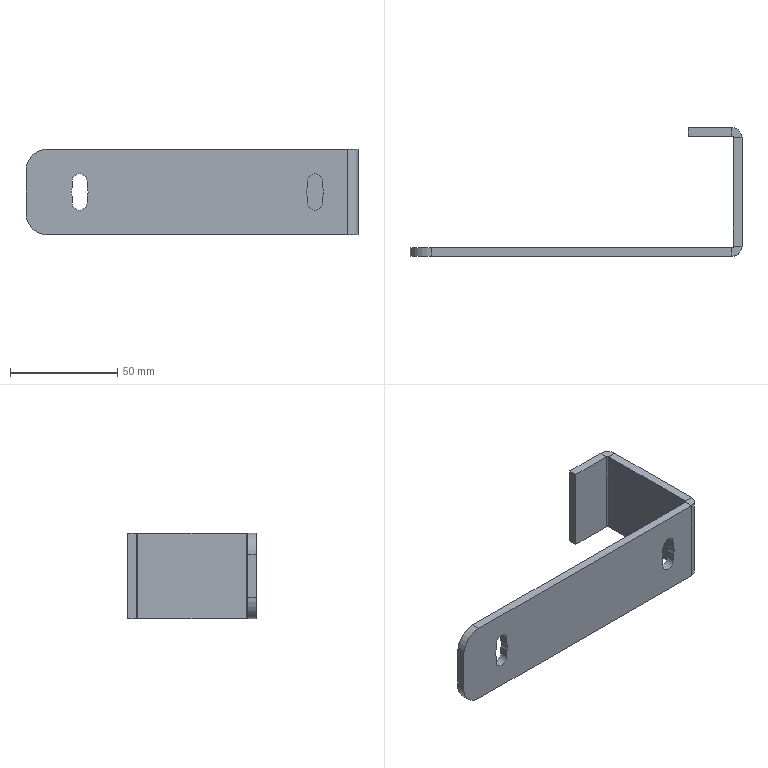Part | SolidWorks | features ICE 2, Fillet 1, FlatPattern 1, SMBaseFlange 1, SheetMetal 1 | 1 solid | 42 faces | box 155 x 60 x 40 mm | volume 35684 mm3 | plane 26 | cylinder 16 | commonest cylinder face diameters 8 x6 7 x4 1.473 x2 9.473 x2 20 x2
STEP:
#1=CARTESIAN_POINT('',(-126.,4.,0.));
#2=VERTEX_POINT('',#1);
#3=CARTESIAN_POINT('',(-126.5,4.,1.936));
#4=VERTEX_POINT('',#3);
#5=CARTESIAN_POINT('',(-130.,4.,0.));
#6=DIRECTION('',(0.,-1.,0.));
#7=DIRECTION('',(1.,0.,0.));
#8=AXIS2_PLACEMENT_3D('',#5,#6,#7);
#9=CIRCLE('',#8,4.);
#10=EDGE_CURVE('',#2,#4,#9,.T.);
#11=ORIENTED_EDGE('',*,*,#10,.F.);
#12=CARTESIAN_POINT('',(-126.,0.,0.));
#13=VERTEX_POINT('',#12);
#14=CARTESIAN_POINT('',(-126.,4.,0.));
#15=DIRECTION('',(0.,-1.,0.));
#16=VECTOR('',#15,1000.);
#17=LINE('',#14,#16);
#18=EDGE_CURVE('',#2,#13,#17,.T.);
#19=ORIENTED_EDGE('',*,*,#18,.T.);
#20=CARTESIAN_POINT('',(-126.5,0.,1.936));
#21=VERTEX_POINT('',#20);
#22=CARTESIAN_POINT('',(-130.,0.,0.));
#23=DIRECTION('',(0.,-1.,0.));
#24=DIRECTION('',(1.,0.,0.));
#25=AXIS2_PLACEMENT_3D('',#22,#23,#24);
#26=CIRCLE('',#25,4.);
#27=EDGE_CURVE('',#13,#21,#26,.T.);
#28=ORIENTED_EDGE('',*,*,#27,.T.);
#29=CARTESIAN_POINT('',(-126.5,4.,1.936));
#30=DIRECTION('',(0.,-1.,0.));
#31=VECTOR('',#30,1000.);
#32=LINE('',#29,#31);
#33=EDGE_CURVE('',#4,#21,#32,.T.);
#34=ORIENTED_EDGE('',*,*,#33,.F.);
#35=EDGE_LOOP('',(#11,#19,#28,#34));
#36=FACE_OUTER_BOUND('',#35,.T.);
#37=CARTESIAN_POINT('',(-130.,4.,0.));
#38=DIRECTION('',(0.,-1.,0.));
#39=DIRECTION('',(1.,0.,0.));
#40=AXIS2_PLACEMENT_3D('',#37,#38,#39);
#41=CYLINDRICAL_SURFACE('',#40,4.);
#42=ADVANCED_FACE('',(#36),#41,.F.);
#43=CARTESIAN_POINT('',(-16.,4.,0.));
#44=VERTEX_POINT('',#43);
#45=CARTESIAN_POINT('',(-16.5,4.,1.936));
#46=VERTEX_POINT('',#45);
#47=CARTESIAN_POINT('',(-20.,4.,0.));
#48=DIRECTION('',(0.,-1.,0.));
#49=DIRECTION('',(1.,0.,0.));
#50=AXIS2_PLACEMENT_3D('',#47,#48,#49);
#51=CIRCLE('',#50,4.);
#52=EDGE_CURVE('',#44,#46,#51,.T.);
#53=ORIENTED_EDGE('',*,*,#52,.F.);
#54=CARTESIAN_POINT('',(-16.,0.,0.));
#55=VERTEX_POINT('',#54);
#56=CARTESIAN_POINT('',(-16.,4.,0.));
#57=DIRECTION('',(0.,-1.,0.));
#58=VECTOR('',#57,1000.);
#59=LINE('',#56,#58);
#60=EDGE_CURVE('',#44,#55,#59,.T.);
#61=ORIENTED_EDGE('',*,*,#60,.T.);
#62=CARTESIAN_POINT('',(-16.5,0.,1.936));
#63=VERTEX_POINT('',#62);
#64=CARTESIAN_POINT('',(-20.,0.,0.));
#65=DIRECTION('',(0.,-1.,0.));
#66=DIRECTION('',(1.,0.,0.));
#67=AXIS2_PLACEMENT_3D('',#64,#65,#66);
#68=CIRCLE('',#67,4.);
#69=EDGE_CURVE('',#55,#63,#68,.T.);
#70=ORIENTED_EDGE('',*,*,#69,.T.);
#71=CARTESIAN_POINT('',(-16.5,4.,1.936));
#72=DIRECTION('',(0.,-1.,0.));
#73=VECTOR('',#72,1000.);
#74=LINE('',#71,#73);
#75=EDGE_CURVE('',#46,#63,#74,.T.);
#76=ORIENTED_EDGE('',*,*,#75,.F.);
#77=EDGE_LOOP('',(#53,#61,#70,#76));
#78=FACE_OUTER_BOUND('',#77,.T.);
#79=CARTESIAN_POINT('',(-20.,4.,0.));
#80=DIRECTION('',(0.,-1.,0.));
#81=DIRECTION('',(1.,0.,0.));
#82=AXIS2_PLACEMENT_3D('',#79,#80,#81);
#83=CYLINDRICAL_SURFACE('',#82,4.);
#84=ADVANCED_FACE('',(#78),#83,.F.);
#85=CARTESIAN_POINT('',(-23.5,4.,1.936));
#86=VERTEX_POINT('',#85);
#87=CARTESIAN_POINT('',(-23.5,4.,-1.936));
#88=VERTEX_POINT('',#87);
#89=CARTESIAN_POINT('',(-20.,4.,0.));
#90=DIRECTION('',(0.,-1.,0.));
#91=DIRECTION('',(1.,0.,0.));
#92=AXIS2_PLACEMENT_3D('',#89,#90,#91);
#93=CIRCLE('',#92,4.);
#94=EDGE_CURVE('',#86,#88,#93,.T.);
#95=ORIENTED_EDGE('',*,*,#94,.T.);
#96=CARTESIAN_POINT('',(-23.5,4.,-5.));
#97=VERTEX_POINT('',#96);
#98=CARTESIAN_POINT('',(-23.5,4.,-5.));
#99=DIRECTION('',(0.,0.,1.));
#100=VECTOR('',#99,1000.);
#101=LINE('',#98,#100);
#102=EDGE_CURVE('',#97,#88,#101,.T.);
#103=ORIENTED_EDGE('',*,*,#102,.F.);
#104=CARTESIAN_POINT('',(-16.5,4.,-5.));
#105=VERTEX_POINT('',#104);
#106=CARTESIAN_POINT('',(-20.,4.,-5.));
#107=DIRECTION('',(0.,1.,0.));
#108=DIRECTION('',(-1.,0.,0.));
#109=AXIS2_PLACEMENT_3D('',#106,#107,#108);
#110=CIRCLE('',#109,3.5);
#111=EDGE_CURVE('',#105,#97,#110,.T.);
#112=ORIENTED_EDGE('',*,*,#111,.F.);
#113=CARTESIAN_POINT('',(-16.5,4.,-1.936));
#114=VERTEX_POINT('',#113);
#115=CARTESIAN_POINT('',(-16.5,4.,-5.));
#116=DIRECTION('',(0.,0.,-1.));
#117=VECTOR('',#116,1000.);
#118=LINE('',#115,#117);
#119=EDGE_CURVE('',#114,#105,#118,.T.);
#120=ORIENTED_EDGE('',*,*,#119,.F.);
#121=CARTESIAN_POINT('',(-20.,4.,0.));
#122=DIRECTION('',(0.,-1.,0.));
#123=DIRECTION('',(1.,0.,0.));
#124=AXIS2_PLACEMENT_3D('',#121,#122,#123);
#125=CIRCLE('',#124,4.);
#126=EDGE_CURVE('',#114,#44,#125,.T.);
#127=ORIENTED_EDGE('',*,*,#126,.T.);
#128=ORIENTED_EDGE('',*,*,#52,.T.);
#129=CARTESIAN_POINT('',(-16.5,4.,5.));
#130=VERTEX_POINT('',#129);
#131=CARTESIAN_POINT('',(-16.5,4.,-5.));
#132=DIRECTION('',(0.,0.,-1.));
#133=VECTOR('',#132,1000.);
#134=LINE('',#131,#133);
#135=EDGE_CURVE('',#130,#46,#134,.T.);
#136=ORIENTED_EDGE('',*,*,#135,.F.);
#137=CARTESIAN_POINT('',(-23.5,4.,5.));
#138=VERTEX_POINT('',#137);
#139=CARTESIAN_POINT('',(-20.,4.,5.));
#140=DIRECTION('',(0.,1.,0.));
#141=DIRECTION('',(-1.,0.,0.));
#142=AXIS2_PLACEMENT_3D('',#139,#140,#141);
#143=CIRCLE('',#142,3.5);
#144=EDGE_CURVE('',#138,#130,#143,.T.);
#145=ORIENTED_EDGE('',*,*,#144,.F.);
#146=CARTESIAN_POINT('',(-23.5,4.,-5.));
#147=DIRECTION('',(0.,0.,1.));
#148=VECTOR('',#147,1000.);
#149=LINE('',#146,#148);
#150=EDGE_CURVE('',#86,#138,#149,.T.);
#151=ORIENTED_EDGE('',*,*,#150,.F.);
#152=EDGE_LOOP('',(#95,#103,#112,#120,#127,#128,#136,#145,#151));
#153=FACE_BOUND('',#152,.T.);
#154=CARTESIAN_POINT('',(-155.,4.,10.));
#155=VERTEX_POINT('',#154);
#156=CARTESIAN_POINT('',(-155.,4.,-10.));
#157=VERTEX_POINT('',#156);
#158=CARTESIAN_POINT('',(-155.,4.,20.));
#159=DIRECTION('',(0.,0.,-1.));
#160=VECTOR('',#159,1000.);
#161=LINE('',#158,#160);
#162=EDGE_CURVE('',#155,#157,#161,.T.);
#163=ORIENTED_EDGE('',*,*,#162,.F.);
#164=CARTESIAN_POINT('',(-145.,4.,20.));
#165=VERTEX_POINT('',#164);
#166=CARTESIAN_POINT('',(-145.,4.,10.));
#167=DIRECTION('',(0.,1.,0.));
#168=DIRECTION('',(1.,0.,0.));
#169=AXIS2_PLACEMENT_3D('',#166,#167,#168);
#170=CIRCLE('',#169,10.);
#171=EDGE_CURVE('',#155,#165,#170,.T.);
#172=ORIENTED_EDGE('',*,*,#171,.T.);
#173=CARTESIAN_POINT('',(-4.737,4.,20.));
#174=VERTEX_POINT('',#173);
#175=CARTESIAN_POINT('',(0.,4.,20.));
#176=DIRECTION('',(-1.,0.,0.));
#177=VECTOR('',#176,1000.);
#178=LINE('',#175,#177);
#179=EDGE_CURVE('',#174,#165,#178,.T.);
#180=ORIENTED_EDGE('',*,*,#179,.F.);
#181=CARTESIAN_POINT('',(-4.737,4.,-20.));
#182=VERTEX_POINT('',#181);
#183=CARTESIAN_POINT('',(-4.737,4.,20.));
#184=DIRECTION('',(0.,0.,-1.));
#185=VECTOR('',#184,1000.);
#186=LINE('',#183,#185);
#187=EDGE_CURVE('',#174,#182,#186,.T.);
#188=ORIENTED_EDGE('',*,*,#187,.T.);
#189=CARTESIAN_POINT('',(-145.,4.,-20.));
#190=VERTEX_POINT('',#189);
#191=CARTESIAN_POINT('',(0.,4.,-20.));
#192=DIRECTION('',(-1.,0.,0.));
#193=VECTOR('',#192,1000.);
#194=LINE('',#191,#193);
#195=EDGE_CURVE('',#182,#190,#194,.T.);
#196=ORIENTED_EDGE('',*,*,#195,.T.);
#197=CARTESIAN_POINT('',(-145.,4.,-10.));
#198=DIRECTION('',(0.,1.,0.));
#199=DIRECTION('',(1.,0.,0.));
#200=AXIS2_PLACEMENT_3D('',#197,#198,#199);
#201=CIRCLE('',#200,10.);
#202=EDGE_CURVE('',#190,#157,#201,.T.);
#203=ORIENTED_EDGE('',*,*,#202,.T.);
#204=EDGE_LOOP('',(#163,#172,#180,#188,#196,#203));
#205=FACE_OUTER_BOUND('',#204,.T.);
#206=CARTESIAN_POINT('',(-126.5,4.,-1.936));
#207=VERTEX_POINT('',#206);
#208=CARTESIAN_POINT('',(-130.,4.,0.));
#209=DIRECTION('',(0.,-1.,0.));
#210=DIRECTION('',(1.,0.,0.));
#211=AXIS2_PLACEMENT_3D('',#208,#209,#210);
#212=CIRCLE('',#211,4.);
#213=EDGE_CURVE('',#207,#2,#212,.T.);
#214=ORIENTED_EDGE('',*,*,#213,.T.);
#215=ORIENTED_EDGE('',*,*,#10,.T.);
#216=CARTESIAN_POINT('',(-126.5,4.,5.));
#217=VERTEX_POINT('',#216);
#218=CARTESIAN_POINT('',(-126.5,4.,-5.));
#219=DIRECTION('',(0.,0.,-1.));
#220=VECTOR('',#219,1000.);
#221=LINE('',#218,#220);
#222=EDGE_CURVE('',#217,#4,#221,.T.);
#223=ORIENTED_EDGE('',*,*,#222,.F.);
#224=CARTESIAN_POINT('',(-133.5,4.,5.));
#225=VERTEX_POINT('',#224);
#226=CARTESIAN_POINT('',(-130.,4.,5.));
#227=DIRECTION('',(0.,1.,0.));
#228=DIRECTION('',(-1.,0.,0.));
#229=AXIS2_PLACEMENT_3D('',#226,#227,#228);
#230=CIRCLE('',#229,3.5);
#231=EDGE_CURVE('',#225,#217,#230,.T.);
#232=ORIENTED_EDGE('',*,*,#231,.F.);
#233=CARTESIAN_POINT('',(-133.5,4.,1.936));
#234=VERTEX_POINT('',#233);
#235=CARTESIAN_POINT('',(-133.5,4.,-5.));
#236=DIRECTION('',(0.,0.,1.));
#237=VECTOR('',#236,1000.);
#238=LINE('',#235,#237);
#239=EDGE_CURVE('',#234,#225,#238,.T.);
#240=ORIENTED_EDGE('',*,*,#239,.F.);
#241=CARTESIAN_POINT('',(-133.5,4.,-1.936));
#242=VERTEX_POINT('',#241);
#243=CARTESIAN_POINT('',(-130.,4.,0.));
#244=DIRECTION('',(0.,-1.,0.));
#245=DIRECTION('',(1.,0.,0.));
#246=AXIS2_PLACEMENT_3D('',#243,#244,#245);
#247=CIRCLE('',#246,4.);
#248=EDGE_CURVE('',#234,#242,#247,.T.);
#249=ORIENTED_EDGE('',*,*,#248,.T.);
#250=CARTESIAN_POINT('',(-133.5,4.,-5.));
#251=VERTEX_POINT('',#250);
#252=CARTESIAN_POINT('',(-133.5,4.,-5.));
#253=DIRECTION('',(0.,0.,1.));
#254=VECTOR('',#253,1000.);
#255=LINE('',#252,#254);
#256=EDGE_CURVE('',#251,#242,#255,.T.);
#257=ORIENTED_EDGE('',*,*,#256,.F.);
#258=CARTESIAN_POINT('',(-126.5,4.,-5.));
#259=VERTEX_POINT('',#258);
#260=CARTESIAN_POINT('',(-130.,4.,-5.));
#261=DIRECTION('',(0.,1.,0.));
#262=DIRECTION('',(-1.,0.,0.));
#263=AXIS2_PLACEMENT_3D('',#260,#261,#262);
#264=CIRCLE('',#263,3.5);
#265=EDGE_CURVE('',#259,#251,#264,.T.);
#266=ORIENTED_EDGE('',*,*,#265,.F.);
#267=CARTESIAN_POINT('',(-126.5,4.,-5.));
#268=DIRECTION('',(0.,0.,-1.));
#269=VECTOR('',#268,1000.);
#270=LINE('',#267,#269);
#271=EDGE_CURVE('',#207,#259,#270,.T.);
#272=ORIENTED_EDGE('',*,*,#271,.F.);
#273=EDGE_LOOP('',(#214,#215,#223,#232,#240,#249,#257,#266,#272));
#274=FACE_BOUND('',#273,.T.);
#275=CARTESIAN_POINT('',(0.,4.,20.));
#276=DIRECTION('',(0.,-1.,0.));
#277=DIRECTION('',(1.,0.,0.));
#278=AXIS2_PLACEMENT_3D('',#275,#276,#277);
#279=PLANE('',#278);
#280=ADVANCED_FACE('',(#153,#205,#274),#279,.F.);
#281=CARTESIAN_POINT('',(-23.5,0.,-1.936));
#282=VERTEX_POINT('',#281);
#283=CARTESIAN_POINT('',(-23.5,0.,-5.));
#284=VERTEX_POINT('',#283);
#285=CARTESIAN_POINT('',(-23.5,0.,20.));
#286=DIRECTION('',(0.,0.,-1.));
#287=VECTOR('',#286,1000.);
#288=LINE('',#285,#287);
#289=EDGE_CURVE('',#282,#284,#288,.T.);
#290=ORIENTED_EDGE('',*,*,#289,.F.);
#291=CARTESIAN_POINT('',(-23.5,0.,1.936));
#292=VERTEX_POINT('',#291);
#293=CARTESIAN_POINT('',(-20.,0.,0.));
#294=DIRECTION('',(0.,-1.,0.));
#295=DIRECTION('',(1.,0.,0.));
#296=AXIS2_PLACEMENT_3D('',#293,#294,#295);
#297=CIRCLE('',#296,4.);
#298=EDGE_CURVE('',#292,#282,#297,.T.);
#299=ORIENTED_EDGE('',*,*,#298,.F.);
#300=CARTESIAN_POINT('',(-23.5,0.,5.));
#301=VERTEX_POINT('',#300);
#302=CARTESIAN_POINT('',(-23.5,0.,20.));
#303=DIRECTION('',(0.,0.,-1.));
#304=VECTOR('',#303,1000.);
#305=LINE('',#302,#304);
#306=EDGE_CURVE('',#301,#292,#305,.T.);
#307=ORIENTED_EDGE('',*,*,#306,.F.);
#308=CARTESIAN_POINT('',(-16.5,0.,5.));
#309=VERTEX_POINT('',#308);
#310=CARTESIAN_POINT('',(-20.,0.,5.));
#311=DIRECTION('',(0.,-1.,0.));
#312=DIRECTION('',(1.,0.,0.));
#313=AXIS2_PLACEMENT_3D('',#310,#311,#312);
#314=CIRCLE('',#313,3.5);
#315=EDGE_CURVE('',#309,#301,#314,.T.);
#316=ORIENTED_EDGE('',*,*,#315,.F.);
#317=CARTESIAN_POINT('',(-16.5,0.,20.));
#318=DIRECTION('',(0.,0.,1.));
#319=VECTOR('',#318,1000.);
#320=LINE('',#317,#319);
#321=EDGE_CURVE('',#63,#309,#320,.T.);
#322=ORIENTED_EDGE('',*,*,#321,.F.);
#323=ORIENTED_EDGE('',*,*,#69,.F.);
#324=CARTESIAN_POINT('',(-16.5,0.,-1.936));
#325=VERTEX_POINT('',#324);
#326=CARTESIAN_POINT('',(-20.,0.,0.));
#327=DIRECTION('',(0.,-1.,0.));
#328=DIRECTION('',(1.,0.,0.));
#329=AXIS2_PLACEMENT_3D('',#326,#327,#328);
#330=CIRCLE('',#329,4.);
#331=EDGE_CURVE('',#325,#55,#330,.T.);
#332=ORIENTED_EDGE('',*,*,#331,.F.);
#333=CARTESIAN_POINT('',(-16.5,0.,-5.));
#334=VERTEX_POINT('',#333);
#335=CARTESIAN_POINT('',(-16.5,0.,20.));
#336=DIRECTION('',(0.,0.,1.));
#337=VECTOR('',#336,1000.);
#338=LINE('',#335,#337);
#339=EDGE_CURVE('',#334,#325,#338,.T.);
#340=ORIENTED_EDGE('',*,*,#339,.F.);
#341=CARTESIAN_POINT('',(-20.,0.,-5.));
#342=DIRECTION('',(0.,-1.,0.));
#343=DIRECTION('',(1.,0.,0.));
#344=AXIS2_PLACEMENT_3D('',#341,#342,#343);
#345=CIRCLE('',#344,3.5);
#346=EDGE_CURVE('',#284,#334,#345,.T.);
#347=ORIENTED_EDGE('',*,*,#346,.F.);
#348=EDGE_LOOP('',(#290,#299,#307,#316,#322,#323,#332,#340,#347));
#349=FACE_BOUND('',#348,.T.);
#350=CARTESIAN_POINT('',(-4.737,0.,20.));
#351=VERTEX_POINT('',#350);
#352=CARTESIAN_POINT('',(-145.,0.,20.));
#353=VERTEX_POINT('',#352);
#354=CARTESIAN_POINT('',(0.,0.,20.));
#355=DIRECTION('',(-1.,0.,0.));
#356=VECTOR('',#355,1000.);
#357=LINE('',#354,#356);
#358=EDGE_CURVE('',#351,#353,#357,.T.);
#359=ORIENTED_EDGE('',*,*,#358,.T.);
#360=CARTESIAN_POINT('',(-155.,0.,10.));
#361=VERTEX_POINT('',#360);
#362=CARTESIAN_POINT('',(-145.,0.,10.));
#363=DIRECTION('',(0.,-1.,0.));
#364=DIRECTION('',(1.,0.,0.));
#365=AXIS2_PLACEMENT_3D('',#362,#363,#364);
#366=CIRCLE('',#365,10.);
#367=EDGE_CURVE('',#353,#361,#366,.T.);
#368=ORIENTED_EDGE('',*,*,#367,.T.);
#369=CARTESIAN_POINT('',(-155.,0.,-10.));
#370=VERTEX_POINT('',#369);
#371=CARTESIAN_POINT('',(-155.,0.,20.));
#372=DIRECTION('',(0.,0.,-1.));
#373=VECTOR('',#372,1000.);
#374=LINE('',#371,#373);
#375=EDGE_CURVE('',#361,#370,#374,.T.);
#376=ORIENTED_EDGE('',*,*,#375,.T.);
#377=CARTESIAN_POINT('',(-145.,0.,-20.));
#378=VERTEX_POINT('',#377);
#379=CARTESIAN_POINT('',(-145.,0.,-10.));
#380=DIRECTION('',(0.,-1.,0.));
#381=DIRECTION('',(1.,0.,0.));
#382=AXIS2_PLACEMENT_3D('',#379,#380,#381);
#383=CIRCLE('',#382,10.);
#384=EDGE_CURVE('',#370,#378,#383,.T.);
#385=ORIENTED_EDGE('',*,*,#384,.T.);
#386=CARTESIAN_POINT('',(-4.737,0.,-20.));
#387=VERTEX_POINT('',#386);
#388=CARTESIAN_POINT('',(0.,0.,-20.));
#389=DIRECTION('',(-1.,0.,0.));
#390=VECTOR('',#389,1000.);
#391=LINE('',#388,#390);
#392=EDGE_CURVE('',#387,#378,#391,.T.);
#393=ORIENTED_EDGE('',*,*,#392,.F.);
#394=CARTESIAN_POINT('',(-4.737,0.,20.));
#395=DIRECTION('',(0.,0.,-1.));
#396=VECTOR('',#395,1000.);
#397=LINE('',#394,#396);
#398=EDGE_CURVE('',#351,#387,#397,.T.);
#399=ORIENTED_EDGE('',*,*,#398,.F.);
#400=EDGE_LOOP('',(#359,#368,#376,#385,#393,#399));
#401=FACE_OUTER_BOUND('',#400,.T.);
#402=CARTESIAN_POINT('',(-126.5,0.,5.));
#403=VERTEX_POINT('',#402);
#404=CARTESIAN_POINT('',(-126.5,0.,20.));
#405=DIRECTION('',(0.,0.,1.));
#406=VECTOR('',#405,1000.);
#407=LINE('',#404,#406);
#408=EDGE_CURVE('',#21,#403,#407,.T.);
#409=ORIENTED_EDGE('',*,*,#408,.F.);
#410=ORIENTED_EDGE('',*,*,#27,.F.);
#411=CARTESIAN_POINT('',(-126.5,0.,-1.936));
#412=VERTEX_POINT('',#411);
#413=CARTESIAN_POINT('',(-130.,0.,0.));
#414=DIRECTION('',(0.,-1.,0.));
#415=DIRECTION('',(1.,0.,0.));
#416=AXIS2_PLACEMENT_3D('',#413,#414,#415);
#417=CIRCLE('',#416,4.);
#418=EDGE_CURVE('',#412,#13,#417,.T.);
#419=ORIENTED_EDGE('',*,*,#418,.F.);
#420=CARTESIAN_POINT('',(-126.5,0.,-5.));
#421=VERTEX_POINT('',#420);
#422=CARTESIAN_POINT('',(-126.5,0.,20.));
#423=DIRECTION('',(0.,0.,1.));
#424=VECTOR('',#423,1000.);
#425=LINE('',#422,#424);
#426=EDGE_CURVE('',#421,#412,#425,.T.);
#427=ORIENTED_EDGE('',*,*,#426,.F.);
#428=CARTESIAN_POINT('',(-133.5,0.,-5.));
#429=VERTEX_POINT('',#428);
#430=CARTESIAN_POINT('',(-130.,0.,-5.));
#431=DIRECTION('',(0.,-1.,0.));
#432=DIRECTION('',(1.,0.,0.));
#433=AXIS2_PLACEMENT_3D('',#430,#431,#432);
#434=CIRCLE('',#433,3.5);
#435=EDGE_CURVE('',#429,#421,#434,.T.);
#436=ORIENTED_EDGE('',*,*,#435,.F.);
#437=CARTESIAN_POINT('',(-133.5,0.,-1.936));
#438=VERTEX_POINT('',#437);
#439=CARTESIAN_POINT('',(-133.5,0.,20.));
#440=DIRECTION('',(0.,0.,-1.));
#441=VECTOR('',#440,1000.);
#442=LINE('',#439,#441);
#443=EDGE_CURVE('',#438,#429,#442,.T.);
#444=ORIENTED_EDGE('',*,*,#443,.F.);
#445=CARTESIAN_POINT('',(-133.5,0.,1.936));
#446=VERTEX_POINT('',#445);
#447=CARTESIAN_POINT('',(-130.,0.,0.));
#448=DIRECTION('',(0.,-1.,0.));
#449=DIRECTION('',(1.,0.,0.));
#450=AXIS2_PLACEMENT_3D('',#447,#448,#449);
#451=CIRCLE('',#450,4.);
#452=EDGE_CURVE('',#446,#438,#451,.T.);
#453=ORIENTED_EDGE('',*,*,#452,.F.);
#454=CARTESIAN_POINT('',(-133.5,0.,5.));
#455=VERTEX_POINT('',#454);
#456=CARTESIAN_POINT('',(-133.5,0.,20.));
#457=DIRECTION('',(0.,0.,-1.));
#458=VECTOR('',#457,1000.);
#459=LINE('',#456,#458);
#460=EDGE_CURVE('',#455,#446,#459,.T.);
#461=ORIENTED_EDGE('',*,*,#460,.F.);
#462=CARTESIAN_POINT('',(-130.,0.,5.));
#463=DIRECTION('',(0.,-1.,0.));
#464=DIRECTION('',(1.,0.,0.));
#465=AXIS2_PLACEMENT_3D('',#462,#463,#464);
#466=CIRCLE('',#465,3.5);
#467=EDGE_CURVE('',#403,#455,#466,.T.);
#468=ORIENTED_EDGE('',*,*,#467,.F.);
#469=EDGE_LOOP('',(#409,#410,#419,#427,#436,#444,#453,#461,#468));
#470=FACE_BOUND('',#469,.T.);
#471=CARTESIAN_POINT('',(0.,0.,20.));
#472=DIRECTION('',(0.,-1.,0.));
#473=DIRECTION('',(1.,0.,0.));
#474=AXIS2_PLACEMENT_3D('',#471,#472,#473);
#475=PLANE('',#474);
#476=ADVANCED_FACE('',(#349,#401,#470),#475,.T.);
#477=ORIENTED_EDGE('',*,*,#33,.T.);
#478=ORIENTED_EDGE('',*,*,#408,.T.);
#479=CARTESIAN_POINT('',(-126.5,-6.,5.));
#480=DIRECTION('',(0.,1.,0.));
#481=VECTOR('',#480,1000.);
#482=LINE('',#479,#481);
#483=EDGE_CURVE('',#403,#217,#482,.T.);
#484=ORIENTED_EDGE('',*,*,#483,.T.);
#485=ORIENTED_EDGE('',*,*,#222,.T.);
#486=EDGE_LOOP('',(#477,#478,#484,#485));
#487=FACE_OUTER_BOUND('',#486,.T.);
#488=CARTESIAN_POINT('',(-126.5,-6.,-5.));
#489=DIRECTION('',(1.,0.,0.));
#490=DIRECTION('',(0.,1.,0.));
#491=AXIS2_PLACEMENT_3D('',#488,#489,#490);
#492=PLANE('',#491);
#493=ADVANCED_FACE('',(#487),#492,.F.);
#494=CARTESIAN_POINT('',(-126.5,4.,-1.936));
#495=DIRECTION('',(0.,-1.,0.));
#496=VECTOR('',#495,1000.);
#497=LINE('',#494,#496);
#498=EDGE_CURVE('',#207,#412,#497,.T.);
#499=ORIENTED_EDGE('',*,*,#498,.F.);
#500=ORIENTED_EDGE('',*,*,#271,.T.);
#501=CARTESIAN_POINT('',(-126.5,-6.,-5.));
#502=DIRECTION('',(0.,1.,0.));
#503=VECTOR('',#502,1000.);
#504=LINE('',#501,#503);
#505=EDGE_CURVE('',#421,#259,#504,.T.);
#506=ORIENTED_EDGE('',*,*,#505,.F.);
#507=ORIENTED_EDGE('',*,*,#426,.T.);
#508=EDGE_LOOP('',(#499,#500,#506,#507));
#509=FACE_OUTER_BOUND('',#508,.T.);
#510=CARTESIAN_POINT('',(-126.5,-6.,-5.));
#511=DIRECTION('',(1.,0.,0.));
#512=DIRECTION('',(0.,1.,0.));
#513=AXIS2_PLACEMENT_3D('',#510,#511,#512);
#514=PLANE('',#513);
#515=ADVANCED_FACE('',(#509),#514,.F.);
#516=CARTESIAN_POINT('',(-23.5,4.,-1.936));
#517=DIRECTION('',(0.,-1.,0.));
#518=VECTOR('',#517,1000.);
#519=LINE('',#516,#518);
#520=EDGE_CURVE('',#88,#282,#519,.T.);
#521=ORIENTED_EDGE('',*,*,#520,.T.);
#522=ORIENTED_EDGE('',*,*,#289,.T.);
#523=CARTESIAN_POINT('',(-23.5,-6.,-5.));
#524=DIRECTION('',(0.,1.,0.));
#525=VECTOR('',#524,1000.);
#526=LINE('',#523,#525);
#527=EDGE_CURVE('',#284,#97,#526,.T.);
#528=ORIENTED_EDGE('',*,*,#527,.T.);
#529=ORIENTED_EDGE('',*,*,#102,.T.);
#530=EDGE_LOOP('',(#521,#522,#528,#529));
#531=FACE_OUTER_BOUND('',#530,.T.);
#532=CARTESIAN_POINT('',(-23.5,-6.,-5.));
#533=DIRECTION('',(-1.,0.,0.));
#534=DIRECTION('',(0.,-1.,0.));
#535=AXIS2_PLACEMENT_3D('',#532,#533,#534);
#536=PLANE('',#535);
#537=ADVANCED_FACE('',(#531),#536,.F.);
#538=CARTESIAN_POINT('',(-23.5,4.,1.936));
#539=DIRECTION('',(0.,-1.,0.));
#540=VECTOR('',#539,1000.);
#541=LINE('',#538,#540);
#542=EDGE_CURVE('',#86,#292,#541,.T.);
#543=ORIENTED_EDGE('',*,*,#542,.F.);
#544=ORIENTED_EDGE('',*,*,#150,.T.);
#545=CARTESIAN_POINT('',(-23.5,-6.,5.));
#546=DIRECTION('',(0.,1.,0.));
#547=VECTOR('',#546,1000.);
#548=LINE('',#545,#547);
#549=EDGE_CURVE('',#301,#138,#548,.T.);
#550=ORIENTED_EDGE('',*,*,#549,.F.);
#551=ORIENTED_EDGE('',*,*,#306,.T.);
#552=EDGE_LOOP('',(#543,#544,#550,#551));
#553=FACE_OUTER_BOUND('',#552,.T.);
#554=CARTESIAN_POINT('',(-23.5,-6.,-5.));
#555=DIRECTION('',(-1.,0.,0.));
#556=DIRECTION('',(0.,-1.,0.));
#557=AXIS2_PLACEMENT_3D('',#554,#555,#556);
#558=PLANE('',#557);
#559=ADVANCED_FACE('',(#553),#558,.F.);
#560=ORIENTED_EDGE('',*,*,#75,.T.);
#561=ORIENTED_EDGE('',*,*,#321,.T.);
#562=CARTESIAN_POINT('',(-16.5,-6.,5.));
#563=DIRECTION('',(0.,1.,0.));
#564=VECTOR('',#563,1000.);
#565=LINE('',#562,#564);
#566=EDGE_CURVE('',#309,#130,#565,.T.);
#567=ORIENTED_EDGE('',*,*,#566,.T.);
#568=ORIENTED_EDGE('',*,*,#135,.T.);
#569=EDGE_LOOP('',(#560,#561,#567,#568));
#570=FACE_OUTER_BOUND('',#569,.T.);
#571=CARTESIAN_POINT('',(-16.5,-6.,-5.));
#572=DIRECTION('',(1.,0.,0.));
#573=DIRECTION('',(0.,1.,0.));
#574=AXIS2_PLACEMENT_3D('',#571,#572,#573);
#575=PLANE('',#574);
#576=ADVANCED_FACE('',(#570),#575,.F.);
#577=CARTESIAN_POINT('',(-16.5,4.,-1.936));
#578=DIRECTION('',(0.,-1.,0.));
#579=VECTOR('',#578,1000.);
#580=LINE('',#577,#579);
#581=EDGE_CURVE('',#114,#325,#580,.T.);
#582=ORIENTED_EDGE('',*,*,#581,.F.);
#583=ORIENTED_EDGE('',*,*,#119,.T.);
#584=CARTESIAN_POINT('',(-16.5,-6.,-5.));
#585=DIRECTION('',(0.,1.,0.));
#586=VECTOR('',#585,1000.);
#587=LINE('',#584,#586);
#588=EDGE_CURVE('',#334,#105,#587,.T.);
#589=ORIENTED_EDGE('',*,*,#588,.F.);
#590=ORIENTED_EDGE('',*,*,#339,.T.);
#591=EDGE_LOOP('',(#582,#583,#589,#590));
#592=FACE_OUTER_BOUND('',#591,.T.);
#593=CARTESIAN_POINT('',(-16.5,-6.,-5.));
#594=DIRECTION('',(1.,0.,0.));
#595=DIRECTION('',(0.,1.,0.));
#596=AXIS2_PLACEMENT_3D('',#593,#594,#595);
#597=PLANE('',#596);
#598=ADVANCED_FACE('',(#592),#597,.F.);
#599=CARTESIAN_POINT('',(-133.5,4.,-1.936));
#600=DIRECTION('',(0.,-1.,0.));
#601=VECTOR('',#600,1000.);
#602=LINE('',#599,#601);
#603=EDGE_CURVE('',#242,#438,#602,.T.);
#604=ORIENTED_EDGE('',*,*,#603,.T.);
#605=ORIENTED_EDGE('',*,*,#443,.T.);
#606=CARTESIAN_POINT('',(-133.5,-6.,-5.));
#607=DIRECTION('',(0.,1.,0.));
#608=VECTOR('',#607,1000.);
#609=LINE('',#606,#608);
#610=EDGE_CURVE('',#429,#251,#609,.T.);
#611=ORIENTED_EDGE('',*,*,#610,.T.);
#612=ORIENTED_EDGE('',*,*,#256,.T.);
#613=EDGE_LOOP('',(#604,#605,#611,#612));
#614=FACE_OUTER_BOUND('',#613,.T.);
#615=CARTESIAN_POINT('',(-133.5,-6.,-5.));
#616=DIRECTION('',(-1.,0.,0.));
#617=DIRECTION('',(0.,-1.,0.));
#618=AXIS2_PLACEMENT_3D('',#615,#616,#617);
#619=PLANE('',#618);
#620=ADVANCED_FACE('',(#614),#619,.F.);
#621=CARTESIAN_POINT('',(-133.5,4.,1.936));
#622=DIRECTION('',(0.,-1.,0.));
#623=VECTOR('',#622,1000.);
#624=LINE('',#621,#623);
#625=EDGE_CURVE('',#234,#446,#624,.T.);
#626=ORIENTED_EDGE('',*,*,#625,.F.);
#627=ORIENTED_EDGE('',*,*,#239,.T.);
#628=CARTESIAN_POINT('',(-133.5,-6.,5.));
#629=DIRECTION('',(0.,1.,0.));
#630=VECTOR('',#629,1000.);
#631=LINE('',#628,#630);
#632=EDGE_CURVE('',#455,#225,#631,.T.);
#633=ORIENTED_EDGE('',*,*,#632,.F.);
#634=ORIENTED_EDGE('',*,*,#460,.T.);
#635=EDGE_LOOP('',(#626,#627,#633,#634));
#636=FACE_OUTER_BOUND('',#635,.T.);
#637=CARTESIAN_POINT('',(-133.5,-6.,-5.));
#638=DIRECTION('',(-1.,0.,0.));
#639=DIRECTION('',(0.,-1.,0.));
#640=AXIS2_PLACEMENT_3D('',#637,#638,#639);
#641=PLANE('',#640);
#642=ADVANCED_FACE('',(#636),#641,.F.);
#643=CARTESIAN_POINT('',(0.,55.263,20.));
#644=VERTEX_POINT('',#643);
#645=CARTESIAN_POINT('',(-4.,55.263,20.));
#646=VERTEX_POINT('',#645);
#647=CARTESIAN_POINT('',(0.,55.263,20.));
#648=DIRECTION('',(-1.,0.,0.));
#649=VECTOR('',#648,1000.);
#650=LINE('',#647,#649);
#651=EDGE_CURVE('',#644,#646,#650,.T.);
#652=ORIENTED_EDGE('',*,*,#651,.F.);
#653=CARTESIAN_POINT('',(-4.737,60.,20.));
#654=VERTEX_POINT('',#653);
#655=CARTESIAN_POINT('',(-4.737,55.263,20.));
#656=DIRECTION('',(0.,0.,-1.));
#657=DIRECTION('',(1.,0.,0.));
#658=AXIS2_PLACEMENT_3D('',#655,#656,#657);
#659=CIRCLE('',#658,4.737);
#660=EDGE_CURVE('',#654,#644,#659,.T.);
#661=ORIENTED_EDGE('',*,*,#660,.F.);
#662=CARTESIAN_POINT('',(-4.737,56.,20.));
#663=VERTEX_POINT('',#662);
#664=CARTESIAN_POINT('',(-4.737,56.,20.));
#665=DIRECTION('',(0.,1.,0.));
#666=VECTOR('',#665,1000.);
#667=LINE('',#664,#666);
#668=EDGE_CURVE('',#663,#654,#667,.T.);
#669=ORIENTED_EDGE('',*,*,#668,.F.);
#670=CARTESIAN_POINT('',(-4.737,55.263,20.));
#671=DIRECTION('',(0.,0.,-1.));
#672=DIRECTION('',(1.,0.,0.));
#673=AXIS2_PLACEMENT_3D('',#670,#671,#672);
#674=CIRCLE('',#673,0.7366);
#675=EDGE_CURVE('',#663,#646,#674,.T.);
#676=ORIENTED_EDGE('',*,*,#675,.T.);
#677=EDGE_LOOP('',(#652,#661,#669,#676));
#678=FACE_OUTER_BOUND('',#677,.T.);
#679=CARTESIAN_POINT('',(0.,55.263,20.));
#680=DIRECTION('',(0.,0.,1.));
#681=DIRECTION('',(1.,0.,0.));
#682=AXIS2_PLACEMENT_3D('',#679,#680,#681);
#683=PLANE('',#682);
#684=ADVANCED_FACE('',(#678),#683,.T.);
#685=CARTESIAN_POINT('',(0.,4.737,20.));
#686=VERTEX_POINT('',#685);
#687=CARTESIAN_POINT('',(0.,60.,20.));
#688=DIRECTION('',(0.,-1.,0.));
#689=VECTOR('',#688,1000.);
#690=LINE('',#687,#689);
#691=EDGE_CURVE('',#644,#686,#690,.T.);
#692=ORIENTED_EDGE('',*,*,#691,.F.);
#693=ORIENTED_EDGE('',*,*,#651,.T.);
#694=CARTESIAN_POINT('',(-4.,4.737,20.));
#695=VERTEX_POINT('',#694);
#696=CARTESIAN_POINT('',(-4.,60.,20.));
#697=DIRECTION('',(0.,-1.,0.));
#698=VECTOR('',#697,1000.);
#699=LINE('',#696,#698);
#700=EDGE_CURVE('',#646,#695,#699,.T.);
#701=ORIENTED_EDGE('',*,*,#700,.T.);
#702=CARTESIAN_POINT('',(-4.,4.737,20.));
#703=DIRECTION('',(1.,0.,0.));
#704=VECTOR('',#703,1000.);
#705=LINE('',#702,#704);
#706=EDGE_CURVE('',#695,#686,#705,.T.);
#707=ORIENTED_EDGE('',*,*,#706,.T.);
#708=EDGE_LOOP('',(#692,#693,#701,#707));
#709=FACE_OUTER_BOUND('',#708,.T.);
#710=CARTESIAN_POINT('',(-4.737,56.,20.));
#711=DIRECTION('',(0.,0.,1.));
#712=DIRECTION('',(1.,0.,0.));
#713=AXIS2_PLACEMENT_3D('',#710,#711,#712);
#714=PLANE('',#713);
#715=ADVANCED_FACE('',(#709),#714,.T.);
#716=CARTESIAN_POINT('',(-4.737,60.,-20.));
#717=VERTEX_POINT('',#716);
#718=CARTESIAN_POINT('',(-4.737,56.,-20.));
#719=VERTEX_POINT('',#718);
#720=CARTESIAN_POINT('',(-4.737,60.,-20.));
#721=DIRECTION('',(0.,-1.,0.));
#722=VECTOR('',#721,1000.);
#723=LINE('',#720,#722);
#724=EDGE_CURVE('',#717,#719,#723,.T.);
#725=ORIENTED_EDGE('',*,*,#724,.F.);
#726=CARTESIAN_POINT('',(0.,55.263,-20.));
#727=VERTEX_POINT('',#726);
#728=CARTESIAN_POINT('',(-4.737,55.263,-20.));
#729=DIRECTION('',(0.,0.,-1.));
#730=DIRECTION('',(1.,0.,0.));
#731=AXIS2_PLACEMENT_3D('',#728,#729,#730);
#732=CIRCLE('',#731,4.737);
#733=EDGE_CURVE('',#717,#727,#732,.T.);
#734=ORIENTED_EDGE('',*,*,#733,.T.);
#735=CARTESIAN_POINT('',(-4.,55.263,-20.));
#736=VERTEX_POINT('',#735);
#737=CARTESIAN_POINT('',(-4.,55.263,-20.));
#738=DIRECTION('',(1.,0.,0.));
#739=VECTOR('',#738,1000.);
#740=LINE('',#737,#739);
#741=EDGE_CURVE('',#736,#727,#740,.T.);
#742=ORIENTED_EDGE('',*,*,#741,.F.);
#743=CARTESIAN_POINT('',(-4.737,55.263,-20.));
#744=DIRECTION('',(0.,0.,-1.));
#745=DIRECTION('',(1.,0.,0.));
#746=AXIS2_PLACEMENT_3D('',#743,#744,#745);
#747=CIRCLE('',#746,0.7366);
#748=EDGE_CURVE('',#719,#736,#747,.T.);
#749=ORIENTED_EDGE('',*,*,#748,.F.);
#750=EDGE_LOOP('',(#725,#734,#742,#749));
#751=FACE_OUTER_BOUND('',#750,.T.);
#752=CARTESIAN_POINT('',(-4.737,60.,-20.));
#753=DIRECTION('',(0.,0.,-1.));
#754=DIRECTION('',(-1.,0.,0.));
#755=AXIS2_PLACEMENT_3D('',#752,#753,#754);
#756=PLANE('',#755);
#757=ADVANCED_FACE('',(#751),#756,.T.);
#758=CARTESIAN_POINT('',(-25.,60.,-20.));
#759=VERTEX_POINT('',#758);
#760=CARTESIAN_POINT('',(-25.,60.,-20.));
#761=DIRECTION('',(1.,0.,0.));
#762=VECTOR('',#761,1000.);
#763=LINE('',#760,#762);
#764=EDGE_CURVE('',#759,#717,#763,.T.);
#765=ORIENTED_EDGE('',*,*,#764,.T.);
#766=ORIENTED_EDGE('',*,*,#724,.T.);
#767=CARTESIAN_POINT('',(-25.,56.,-20.));
#768=VERTEX_POINT('',#767);
#769=CARTESIAN_POINT('',(-25.,56.,-20.));
#770=DIRECTION('',(1.,0.,0.));
#771=VECTOR('',#770,1000.);
#772=LINE('',#769,#771);
#773=EDGE_CURVE('',#768,#719,#772,.T.);
#774=ORIENTED_EDGE('',*,*,#773,.F.);
#775=CARTESIAN_POINT('',(-25.,56.,-20.));
#776=DIRECTION('',(0.,1.,0.));
#777=VECTOR('',#776,1000.);
#778=LINE('',#775,#777);
#779=EDGE_CURVE('',#768,#759,#778,.T.);
#780=ORIENTED_EDGE('',*,*,#779,.T.);
#781=EDGE_LOOP('',(#765,#766,#774,#780));
#782=FACE_OUTER_BOUND('',#781,.T.);
#783=CARTESIAN_POINT('',(-4.,55.263,-20.));
#784=DIRECTION('',(0.,0.,-1.));
#785=DIRECTION('',(-1.,0.,0.));
#786=AXIS2_PLACEMENT_3D('',#783,#784,#785);
#787=PLANE('',#786);
#788=ADVANCED_FACE('',(#782),#787,.T.);
#789=CARTESIAN_POINT('',(-4.737,0.,20.));
#790=DIRECTION('',(0.,1.,0.));
#791=VECTOR('',#790,1000.);
#792=LINE('',#789,#791);
#793=EDGE_CURVE('',#351,#174,#792,.T.);
#794=ORIENTED_EDGE('',*,*,#793,.F.);
#795=CARTESIAN_POINT('',(-4.737,4.737,20.));
#796=DIRECTION('',(0.,0.,-1.));
#797=DIRECTION('',(1.,0.,0.));
#798=AXIS2_PLACEMENT_3D('',#795,#796,#797);
#799=CIRCLE('',#798,4.737);
#800=EDGE_CURVE('',#686,#351,#799,.T.);
#801=ORIENTED_EDGE('',*,*,#800,.F.);
#802=ORIENTED_EDGE('',*,*,#706,.F.);
#803=CARTESIAN_POINT('',(-4.737,4.737,20.));
#804=DIRECTION('',(0.,0.,-1.));
#805=DIRECTION('',(1.,0.,0.));
#806=AXIS2_PLACEMENT_3D('',#803,#804,#805);
#807=CIRCLE('',#806,0.7366);
#808=EDGE_CURVE('',#695,#174,#807,.T.);
#809=ORIENTED_EDGE('',*,*,#808,.T.);
#810=EDGE_LOOP('',(#794,#801,#802,#809));
#811=FACE_OUTER_BOUND('',#810,.T.);
#812=CARTESIAN_POINT('',(-4.737,0.,20.));
#813=DIRECTION('',(0.,0.,1.));
#814=DIRECTION('',(1.,0.,0.));
#815=AXIS2_PLACEMENT_3D('',#812,#813,#814);
#816=PLANE('',#815);
#817=ADVANCED_FACE('',(#811),#816,.T.);
#818=ORIENTED_EDGE('',*,*,#179,.T.);
#819=CARTESIAN_POINT('',(-145.,4.737,20.));
#820=DIRECTION('',(0.,-1.,0.));
#821=VECTOR('',#820,1000.);
#822=LINE('',#819,#821);
#823=EDGE_CURVE('',#165,#353,#822,.T.);
#824=ORIENTED_EDGE('',*,*,#823,.T.);
#825=ORIENTED_EDGE('',*,*,#358,.F.);
#826=ORIENTED_EDGE('',*,*,#793,.T.);
#827=EDGE_LOOP('',(#818,#824,#825,#826));
#828=FACE_OUTER_BOUND('',#827,.T.);
#829=CARTESIAN_POINT('',(-4.,4.737,20.));
#830=DIRECTION('',(0.,0.,1.));
#831=DIRECTION('',(1.,0.,0.));
#832=AXIS2_PLACEMENT_3D('',#829,#830,#831);
#833=PLANE('',#832);
#834=ADVANCED_FACE('',(#828),#833,.T.);
#835=CARTESIAN_POINT('',(0.,4.737,-20.));
#836=VERTEX_POINT('',#835);
#837=CARTESIAN_POINT('',(-4.,4.737,-20.));
#838=VERTEX_POINT('',#837);
#839=CARTESIAN_POINT('',(0.,4.737,-20.));
#840=DIRECTION('',(-1.,0.,0.));
#841=VECTOR('',#840,1000.);
#842=LINE('',#839,#841);
#843=EDGE_CURVE('',#836,#838,#842,.T.);
#844=ORIENTED_EDGE('',*,*,#843,.F.);
#845=CARTESIAN_POINT('',(-4.737,4.737,-20.));
#846=DIRECTION('',(0.,0.,-1.));
#847=DIRECTION('',(1.,0.,0.));
#848=AXIS2_PLACEMENT_3D('',#845,#846,#847);
#849=CIRCLE('',#848,4.737);
#850=EDGE_CURVE('',#836,#387,#849,.T.);
#851=ORIENTED_EDGE('',*,*,#850,.T.);
#852=CARTESIAN_POINT('',(-4.737,4.,-20.));
#853=DIRECTION('',(0.,-1.,0.));
#854=VECTOR('',#853,1000.);
#855=LINE('',#852,#854);
#856=EDGE_CURVE('',#182,#387,#855,.T.);
#857=ORIENTED_EDGE('',*,*,#856,.F.);
#858=CARTESIAN_POINT('',(-4.737,4.737,-20.));
#859=DIRECTION('',(0.,0.,-1.));
#860=DIRECTION('',(1.,0.,0.));
#861=AXIS2_PLACEMENT_3D('',#858,#859,#860);
#862=CIRCLE('',#861,0.7366);
#863=EDGE_CURVE('',#838,#182,#862,.T.);
#864=ORIENTED_EDGE('',*,*,#863,.F.);
#865=EDGE_LOOP('',(#844,#851,#857,#864));
#866=FACE_OUTER_BOUND('',#865,.T.);
#867=CARTESIAN_POINT('',(0.,4.737,-20.));
#868=DIRECTION('',(0.,0.,-1.));
#869=DIRECTION('',(-1.,0.,0.));
#870=AXIS2_PLACEMENT_3D('',#867,#868,#869);
#871=PLANE('',#870);
#872=ADVANCED_FACE('',(#866),#871,.T.);
#873=CARTESIAN_POINT('',(0.,60.,-20.));
#874=DIRECTION('',(0.,-1.,0.));
#875=VECTOR('',#874,1000.);
#876=LINE('',#873,#875);
#877=EDGE_CURVE('',#727,#836,#876,.T.);
#878=ORIENTED_EDGE('',*,*,#877,.T.);
#879=ORIENTED_EDGE('',*,*,#843,.T.);
#880=CARTESIAN_POINT('',(-4.,60.,-20.));
#881=DIRECTION('',(0.,-1.,0.));
#882=VECTOR('',#881,1000.);
#883=LINE('',#880,#882);
#884=EDGE_CURVE('',#736,#838,#883,.T.);
#885=ORIENTED_EDGE('',*,*,#884,.F.);
#886=ORIENTED_EDGE('',*,*,#741,.T.);
#887=EDGE_LOOP('',(#878,#879,#885,#886));
#888=FACE_OUTER_BOUND('',#887,.T.);
#889=CARTESIAN_POINT('',(-4.737,4.,-20.));
#890=DIRECTION('',(0.,0.,-1.));
#891=DIRECTION('',(-1.,0.,0.));
#892=AXIS2_PLACEMENT_3D('',#889,#890,#891);
#893=PLANE('',#892);
#894=ADVANCED_FACE('',(#888),#893,.T.);
#895=ORIENTED_EDGE('',*,*,#375,.F.);
#896=CARTESIAN_POINT('',(-155.,0.,10.));
#897=DIRECTION('',(0.,1.,0.));
#898=VECTOR('',#897,1000.);
#899=LINE('',#896,#898);
#900=EDGE_CURVE('',#361,#155,#899,.T.);
#901=ORIENTED_EDGE('',*,*,#900,.T.);
#902=ORIENTED_EDGE('',*,*,#162,.T.);
#903=CARTESIAN_POINT('',(-155.,0.,-10.));
#904=DIRECTION('',(0.,-1.,0.));
#905=VECTOR('',#904,1000.);
#906=LINE('',#903,#905);
#907=EDGE_CURVE('',#157,#370,#906,.T.);
#908=ORIENTED_EDGE('',*,*,#907,.T.);
#909=EDGE_LOOP('',(#895,#901,#902,#908));
#910=FACE_OUTER_BOUND('',#909,.T.);
#911=CARTESIAN_POINT('',(-155.,0.,20.));
#912=DIRECTION('',(-1.,0.,0.));
#913=DIRECTION('',(0.,0.,1.));
#914=AXIS2_PLACEMENT_3D('',#911,#912,#913);
#915=PLANE('',#914);
#916=ADVANCED_FACE('',(#910),#915,.T.);
#917=ORIENTED_EDGE('',*,*,#850,.F.);
#918=CARTESIAN_POINT('',(0.,4.737,20.));
#919=DIRECTION('',(0.,0.,-1.));
#920=VECTOR('',#919,1000.);
#921=LINE('',#918,#920);
#922=EDGE_CURVE('',#686,#836,#921,.T.);
#923=ORIENTED_EDGE('',*,*,#922,.F.);
#924=ORIENTED_EDGE('',*,*,#800,.T.);
#925=ORIENTED_EDGE('',*,*,#398,.T.);
#926=EDGE_LOOP('',(#917,#923,#924,#925));
#927=FACE_OUTER_BOUND('',#926,.T.);
#928=CARTESIAN_POINT('',(-4.737,4.737,20.));
#929=DIRECTION('',(0.,0.,-1.));
#930=DIRECTION('',(-1.,0.,0.));
#931=AXIS2_PLACEMENT_3D('',#928,#929,#930);
#932=CYLINDRICAL_SURFACE('',#931,4.737);
#933=ADVANCED_FACE('',(#927),#932,.T.);
#934=ORIENTED_EDGE('',*,*,#877,.F.);
#935=CARTESIAN_POINT('',(0.,55.263,20.));
#936=DIRECTION('',(0.,0.,-1.));
#937=VECTOR('',#936,1000.);
#938=LINE('',#935,#937);
#939=EDGE_CURVE('',#644,#727,#938,.T.);
#940=ORIENTED_EDGE('',*,*,#939,.F.);
#941=ORIENTED_EDGE('',*,*,#691,.T.);
#942=ORIENTED_EDGE('',*,*,#922,.T.);
#943=EDGE_LOOP('',(#934,#940,#941,#942));
#944=FACE_OUTER_BOUND('',#943,.T.);
#945=CARTESIAN_POINT('',(0.,60.,20.));
#946=DIRECTION('',(1.,0.,0.));
#947=DIRECTION('',(0.,1.,0.));
#948=AXIS2_PLACEMENT_3D('',#945,#946,#947);
#949=PLANE('',#948);
#950=ADVANCED_FACE('',(#944),#949,.T.);
#951=ORIENTED_EDGE('',*,*,#733,.F.);
#952=CARTESIAN_POINT('',(-4.737,60.,20.));
#953=DIRECTION('',(0.,0.,-1.));
#954=VECTOR('',#953,1000.);
#955=LINE('',#952,#954);
#956=EDGE_CURVE('',#654,#717,#955,.T.);
#957=ORIENTED_EDGE('',*,*,#956,.F.);
#958=ORIENTED_EDGE('',*,*,#660,.T.);
#959=ORIENTED_EDGE('',*,*,#939,.T.);
#960=EDGE_LOOP('',(#951,#957,#958,#959));
#961=FACE_OUTER_BOUND('',#960,.T.);
#962=CARTESIAN_POINT('',(-4.737,55.263,20.));
#963=DIRECTION('',(0.,0.,-1.));
#964=DIRECTION('',(-1.,0.,0.));
#965=AXIS2_PLACEMENT_3D('',#962,#963,#964);
#966=CYLINDRICAL_SURFACE('',#965,4.737);
#967=ADVANCED_FACE('',(#961),#966,.T.);
#968=ORIENTED_EDGE('',*,*,#764,.F.);
#969=CARTESIAN_POINT('',(-25.,60.,20.));
#970=VERTEX_POINT('',#969);
#971=CARTESIAN_POINT('',(-25.,60.,20.));
#972=DIRECTION('',(0.,0.,-1.));
#973=VECTOR('',#972,1000.);
#974=LINE('',#971,#973);
#975=EDGE_CURVE('',#970,#759,#974,.T.);
#976=ORIENTED_EDGE('',*,*,#975,.F.);
#977=CARTESIAN_POINT('',(-25.,60.,20.));
#978=DIRECTION('',(1.,0.,0.));
#979=VECTOR('',#978,1000.);
#980=LINE('',#977,#979);
#981=EDGE_CURVE('',#970,#654,#980,.T.);
#982=ORIENTED_EDGE('',*,*,#981,.T.);
#983=ORIENTED_EDGE('',*,*,#956,.T.);
#984=EDGE_LOOP('',(#968,#976,#982,#983));
#985=FACE_OUTER_BOUND('',#984,.T.);
#986=CARTESIAN_POINT('',(-25.,60.,20.));
#987=DIRECTION('',(0.,1.,0.));
#988=DIRECTION('',(0.,0.,1.));
#989=AXIS2_PLACEMENT_3D('',#986,#987,#988);
#990=PLANE('',#989);
#991=ADVANCED_FACE('',(#985),#990,.T.);
#992=ORIENTED_EDGE('',*,*,#779,.F.);
#993=CARTESIAN_POINT('',(-25.,56.,20.));
#994=VERTEX_POINT('',#993);
#995=CARTESIAN_POINT('',(-25.,56.,20.));
#996=DIRECTION('',(0.,0.,-1.));
#997=VECTOR('',#996,1000.);
#998=LINE('',#995,#997);
#999=EDGE_CURVE('',#994,#768,#998,.T.);
#1000=ORIENTED_EDGE('',*,*,#999,.F.);
#1001=CARTESIAN_POINT('',(-25.,56.,20.));
#1002=DIRECTION('',(0.,1.,0.));
#1003=VECTOR('',#1002,1000.);
#1004=LINE('',#1001,#1003);
#1005=EDGE_CURVE('',#994,#970,#1004,.T.);
#1006=ORIENTED_EDGE('',*,*,#1005,.T.);
#1007=ORIENTED_EDGE('',*,*,#975,.T.);
#1008=EDGE_LOOP('',(#992,#1000,#1006,#1007));
#1009=FACE_OUTER_BOUND('',#1008,.T.);
#1010=CARTESIAN_POINT('',(-25.,56.,20.));
#1011=DIRECTION('',(-1.,0.,0.));
#1012=DIRECTION('',(0.,0.,1.));
#1013=AXIS2_PLACEMENT_3D('',#1010,#1011,#1012);
#1014=PLANE('',#1013);
#1015=ADVANCED_FACE('',(#1009),#1014,.T.);
#1016=ORIENTED_EDGE('',*,*,#773,.T.);
#1017=CARTESIAN_POINT('',(-4.737,56.,20.));
#1018=DIRECTION('',(0.,0.,-1.));
#1019=VECTOR('',#1018,1000.);
#1020=LINE('',#1017,#1019);
#1021=EDGE_CURVE('',#663,#719,#1020,.T.);
#1022=ORIENTED_EDGE('',*,*,#1021,.F.);
#1023=CARTESIAN_POINT('',(-25.,56.,20.));
#1024=DIRECTION('',(1.,0.,0.));
#1025=VECTOR('',#1024,1000.);
#1026=LINE('',#1023,#1025);
#1027=EDGE_CURVE('',#994,#663,#1026,.T.);
#1028=ORIENTED_EDGE('',*,*,#1027,.F.);
#1029=ORIENTED_EDGE('',*,*,#999,.T.);
#1030=EDGE_LOOP('',(#1016,#1022,#1028,#1029));
#1031=FACE_OUTER_BOUND('',#1030,.T.);
#1032=CARTESIAN_POINT('',(-25.,56.,20.));
#1033=DIRECTION('',(0.,1.,0.));
#1034=DIRECTION('',(0.,0.,1.));
#1035=AXIS2_PLACEMENT_3D('',#1032,#1033,#1034);
#1036=PLANE('',#1035);
#1037=ADVANCED_FACE('',(#1031),#1036,.F.);
#1038=ORIENTED_EDGE('',*,*,#748,.T.);
#1039=CARTESIAN_POINT('',(-4.,55.263,20.));
#1040=DIRECTION('',(0.,0.,-1.));
#1041=VECTOR('',#1040,1000.);
#1042=LINE('',#1039,#1041);
#1043=EDGE_CURVE('',#646,#736,#1042,.T.);
#1044=ORIENTED_EDGE('',*,*,#1043,.F.);
#1045=ORIENTED_EDGE('',*,*,#675,.F.);
#1046=ORIENTED_EDGE('',*,*,#1021,.T.);
#1047=EDGE_LOOP('',(#1038,#1044,#1045,#1046));
#1048=FACE_OUTER_BOUND('',#1047,.T.);
#1049=CARTESIAN_POINT('',(-4.737,55.263,20.));
#1050=DIRECTION('',(0.,0.,-1.));
#1051=DIRECTION('',(-1.,0.,0.));
#1052=AXIS2_PLACEMENT_3D('',#1049,#1050,#1051);
#1053=CYLINDRICAL_SURFACE('',#1052,0.7366);
#1054=ADVANCED_FACE('',(#1048),#1053,.F.);
#1055=ORIENTED_EDGE('',*,*,#884,.T.);
#1056=CARTESIAN_POINT('',(-4.,4.737,20.));
#1057=DIRECTION('',(0.,0.,-1.));
#1058=VECTOR('',#1057,1000.);
#1059=LINE('',#1056,#1058);
#1060=EDGE_CURVE('',#695,#838,#1059,.T.);
#1061=ORIENTED_EDGE('',*,*,#1060,.F.);
#1062=ORIENTED_EDGE('',*,*,#700,.F.);
#1063=ORIENTED_EDGE('',*,*,#1043,.T.);
#1064=EDGE_LOOP('',(#1055,#1061,#1062,#1063));
#1065=FACE_OUTER_BOUND('',#1064,.T.);
#1066=CARTESIAN_POINT('',(-4.,60.,20.));
#1067=DIRECTION('',(1.,0.,0.));
#1068=DIRECTION('',(0.,1.,0.));
#1069=AXIS2_PLACEMENT_3D('',#1066,#1067,#1068);
#1070=PLANE('',#1069);
#1071=ADVANCED_FACE('',(#1065),#1070,.F.);
#1072=ORIENTED_EDGE('',*,*,#863,.T.);
#1073=ORIENTED_EDGE('',*,*,#187,.F.);
#1074=ORIENTED_EDGE('',*,*,#808,.F.);
#1075=ORIENTED_EDGE('',*,*,#1060,.T.);
#1076=EDGE_LOOP('',(#1072,#1073,#1074,#1075));
#1077=FACE_OUTER_BOUND('',#1076,.T.);
#1078=CARTESIAN_POINT('',(-4.737,4.737,20.));
#1079=DIRECTION('',(0.,0.,-1.));
#1080=DIRECTION('',(-1.,0.,0.));
#1081=AXIS2_PLACEMENT_3D('',#1078,#1079,#1080);
#1082=CYLINDRICAL_SURFACE('',#1081,0.7366);
#1083=ADVANCED_FACE('',(#1077),#1082,.F.);
#1084=ORIENTED_EDGE('',*,*,#1027,.T.);
#1085=ORIENTED_EDGE('',*,*,#668,.T.);
#1086=ORIENTED_EDGE('',*,*,#981,.F.);
#1087=ORIENTED_EDGE('',*,*,#1005,.F.);
#1088=EDGE_LOOP('',(#1084,#1085,#1086,#1087));
#1089=FACE_OUTER_BOUND('',#1088,.T.);
#1090=CARTESIAN_POINT('',(-4.737,4.737,20.));
#1091=DIRECTION('',(0.,0.,1.));
#1092=DIRECTION('',(1.,0.,0.));
#1093=AXIS2_PLACEMENT_3D('',#1090,#1091,#1092);
#1094=PLANE('',#1093);
#1095=ADVANCED_FACE('',(#1089),#1094,.T.);
#1096=ORIENTED_EDGE('',*,*,#392,.T.);
#1097=CARTESIAN_POINT('',(-145.,4.,-20.));
#1098=DIRECTION('',(0.,1.,0.));
#1099=VECTOR('',#1098,1000.);
#1100=LINE('',#1097,#1099);
#1101=EDGE_CURVE('',#378,#190,#1100,.T.);
#1102=ORIENTED_EDGE('',*,*,#1101,.T.);
#1103=ORIENTED_EDGE('',*,*,#195,.F.);
#1104=ORIENTED_EDGE('',*,*,#856,.T.);
#1105=EDGE_LOOP('',(#1096,#1102,#1103,#1104));
#1106=FACE_OUTER_BOUND('',#1105,.T.);
#1107=CARTESIAN_POINT('',(-4.737,4.737,-20.));
#1108=DIRECTION('',(0.,0.,1.));
#1109=DIRECTION('',(1.,0.,0.));
#1110=AXIS2_PLACEMENT_3D('',#1107,#1108,#1109);
#1111=PLANE('',#1110);
#1112=ADVANCED_FACE('',(#1106),#1111,.F.);
#1113=ORIENTED_EDGE('',*,*,#435,.T.);
#1114=ORIENTED_EDGE('',*,*,#505,.T.);
#1115=ORIENTED_EDGE('',*,*,#265,.T.);
#1116=ORIENTED_EDGE('',*,*,#610,.F.);
#1117=EDGE_LOOP('',(#1113,#1114,#1115,#1116));
#1118=FACE_OUTER_BOUND('',#1117,.T.);
#1119=CARTESIAN_POINT('',(-130.,-6.,-5.));
#1120=DIRECTION('',(0.,1.,0.));
#1121=DIRECTION('',(-1.,0.,0.));
#1122=AXIS2_PLACEMENT_3D('',#1119,#1120,#1121);
#1123=CYLINDRICAL_SURFACE('',#1122,3.5);
#1124=ADVANCED_FACE('',(#1118),#1123,.F.);
#1125=ORIENTED_EDGE('',*,*,#467,.T.);
#1126=ORIENTED_EDGE('',*,*,#632,.T.);
#1127=ORIENTED_EDGE('',*,*,#231,.T.);
#1128=ORIENTED_EDGE('',*,*,#483,.F.);
#1129=EDGE_LOOP('',(#1125,#1126,#1127,#1128));
#1130=FACE_OUTER_BOUND('',#1129,.T.);
#1131=CARTESIAN_POINT('',(-130.,-6.,5.));
#1132=DIRECTION('',(0.,1.,0.));
#1133=DIRECTION('',(-1.,0.,0.));
#1134=AXIS2_PLACEMENT_3D('',#1131,#1132,#1133);
#1135=CYLINDRICAL_SURFACE('',#1134,3.5);
#1136=ADVANCED_FACE('',(#1130),#1135,.F.);
#1137=ORIENTED_EDGE('',*,*,#346,.T.);
#1138=ORIENTED_EDGE('',*,*,#588,.T.);
#1139=ORIENTED_EDGE('',*,*,#111,.T.);
#1140=ORIENTED_EDGE('',*,*,#527,.F.);
#1141=EDGE_LOOP('',(#1137,#1138,#1139,#1140));
#1142=FACE_OUTER_BOUND('',#1141,.T.);
#1143=CARTESIAN_POINT('',(-20.,-6.,-5.));
#1144=DIRECTION('',(0.,1.,0.));
#1145=DIRECTION('',(-1.,0.,0.));
#1146=AXIS2_PLACEMENT_3D('',#1143,#1144,#1145);
#1147=CYLINDRICAL_SURFACE('',#1146,3.5);
#1148=ADVANCED_FACE('',(#1142),#1147,.F.);
#1149=ORIENTED_EDGE('',*,*,#315,.T.);
#1150=ORIENTED_EDGE('',*,*,#549,.T.);
#1151=ORIENTED_EDGE('',*,*,#144,.T.);
#1152=ORIENTED_EDGE('',*,*,#566,.F.);
#1153=EDGE_LOOP('',(#1149,#1150,#1151,#1152));
#1154=FACE_OUTER_BOUND('',#1153,.T.);
#1155=CARTESIAN_POINT('',(-20.,-6.,5.));
#1156=DIRECTION('',(0.,1.,0.));
#1157=DIRECTION('',(-1.,0.,0.));
#1158=AXIS2_PLACEMENT_3D('',#1155,#1156,#1157);
#1159=CYLINDRICAL_SURFACE('',#1158,3.5);
#1160=ADVANCED_FACE('',(#1154),#1159,.F.);
#1161=ORIENTED_EDGE('',*,*,#367,.F.);
#1162=ORIENTED_EDGE('',*,*,#823,.F.);
#1163=ORIENTED_EDGE('',*,*,#171,.F.);
#1164=ORIENTED_EDGE('',*,*,#900,.F.);
#1165=EDGE_LOOP('',(#1161,#1162,#1163,#1164));
#1166=FACE_OUTER_BOUND('',#1165,.T.);
#1167=CARTESIAN_POINT('',(-145.,0.,10.));
#1168=DIRECTION('',(0.,1.,0.));
#1169=DIRECTION('',(0.,0.,1.));
#1170=AXIS2_PLACEMENT_3D('',#1167,#1168,#1169);
#1171=CYLINDRICAL_SURFACE('',#1170,10.);
#1172=ADVANCED_FACE('',(#1166),#1171,.T.);
#1173=ORIENTED_EDGE('',*,*,#384,.F.);
#1174=ORIENTED_EDGE('',*,*,#907,.F.);
#1175=ORIENTED_EDGE('',*,*,#202,.F.);
#1176=ORIENTED_EDGE('',*,*,#1101,.F.);
#1177=EDGE_LOOP('',(#1173,#1174,#1175,#1176));
#1178=FACE_OUTER_BOUND('',#1177,.T.);
#1179=CARTESIAN_POINT('',(-145.,4.737,-10.));
#1180=DIRECTION('',(0.,-1.,0.));
#1181=DIRECTION('',(0.,0.,-1.));
#1182=AXIS2_PLACEMENT_3D('',#1179,#1180,#1181);
#1183=CYLINDRICAL_SURFACE('',#1182,10.);
#1184=ADVANCED_FACE('',(#1178),#1183,.T.);
#1185=ORIENTED_EDGE('',*,*,#603,.F.);
#1186=ORIENTED_EDGE('',*,*,#248,.F.);
#1187=ORIENTED_EDGE('',*,*,#625,.T.);
#1188=ORIENTED_EDGE('',*,*,#452,.T.);
#1189=EDGE_LOOP('',(#1185,#1186,#1187,#1188));
#1190=FACE_OUTER_BOUND('',#1189,.T.);
#1191=CARTESIAN_POINT('',(-130.,4.,0.));
#1192=DIRECTION('',(0.,-1.,0.));
#1193=DIRECTION('',(1.,0.,0.));
#1194=AXIS2_PLACEMENT_3D('',#1191,#1192,#1193);
#1195=CYLINDRICAL_SURFACE('',#1194,4.);
#1196=ADVANCED_FACE('',(#1190),#1195,.F.);
#1197=ORIENTED_EDGE('',*,*,#60,.F.);
#1198=ORIENTED_EDGE('',*,*,#126,.F.);
#1199=ORIENTED_EDGE('',*,*,#581,.T.);
#1200=ORIENTED_EDGE('',*,*,#331,.T.);
#1201=EDGE_LOOP('',(#1197,#1198,#1199,#1200));
#1202=FACE_OUTER_BOUND('',#1201,.T.);
#1203=CARTESIAN_POINT('',(-20.,4.,0.));
#1204=DIRECTION('',(0.,-1.,0.));
#1205=DIRECTION('',(1.,0.,0.));
#1206=AXIS2_PLACEMENT_3D('',#1203,#1204,#1205);
#1207=CYLINDRICAL_SURFACE('',#1206,4.);
#1208=ADVANCED_FACE('',(#1202),#1207,.F.);
#1209=ORIENTED_EDGE('',*,*,#520,.F.);
#1210=ORIENTED_EDGE('',*,*,#94,.F.);
#1211=ORIENTED_EDGE('',*,*,#542,.T.);
#1212=ORIENTED_EDGE('',*,*,#298,.T.);
#1213=EDGE_LOOP('',(#1209,#1210,#1211,#1212));
#1214=FACE_OUTER_BOUND('',#1213,.T.);
#1215=CARTESIAN_POINT('',(-20.,4.,0.));
#1216=DIRECTION('',(0.,-1.,0.));
#1217=DIRECTION('',(1.,0.,0.));
#1218=AXIS2_PLACEMENT_3D('',#1215,#1216,#1217);
#1219=CYLINDRICAL_SURFACE('',#1218,4.);
#1220=ADVANCED_FACE('',(#1214),#1219,.F.);
#1221=ORIENTED_EDGE('',*,*,#18,.F.);
#1222=ORIENTED_EDGE('',*,*,#213,.F.);
#1223=ORIENTED_EDGE('',*,*,#498,.T.);
#1224=ORIENTED_EDGE('',*,*,#418,.T.);
#1225=EDGE_LOOP('',(#1221,#1222,#1223,#1224));
#1226=FACE_OUTER_BOUND('',#1225,.T.);
#1227=CARTESIAN_POINT('',(-130.,4.,0.));
#1228=DIRECTION('',(0.,-1.,0.));
#1229=DIRECTION('',(1.,0.,0.));
#1230=AXIS2_PLACEMENT_3D('',#1227,#1228,#1229);
#1231=CYLINDRICAL_SURFACE('',#1230,4.);
#1232=ADVANCED_FACE('',(#1226),#1231,.F.);
#1233=CLOSED_SHELL('',(#42,#84,#280,#476,#493,#515,#537,#559,#576,#598,#620,#642,#684,#715,#757,#788,#817,#834,#872,#894,#916,#933,#950,#967,#991,#1015,#1037,#1054,#1071,#1083,#1095,#1112,#1124,#1136,#1148,#1160,#1172,#1184,#1196,#1208,#1220,#1232));
#1234=MANIFOLD_SOLID_BREP('',#1233);
#1235=CARTESIAN_POINT('',(0.,0.,0.));
#1236=DIRECTION('',(0.,0.,1.));
#1237=DIRECTION('',(1.,0.,0.));
#1238=AXIS2_PLACEMENT_3D('',#1235,#1236,#1237);
#1239=(LENGTH_UNIT()NAMED_UNIT(*)SI_UNIT(.MILLI.,.METRE.));
#1240=UNCERTAINTY_MEASURE_WITH_UNIT(LENGTH_MEASURE(0.00001),#1239,'','');
#1241=(NAMED_UNIT(*)PLANE_ANGLE_UNIT()SI_UNIT($,.RADIAN.));
#1242=(NAMED_UNIT(*)SI_UNIT($,.STERADIAN.)SOLID_ANGLE_UNIT());
#1243=(GEOMETRIC_REPRESENTATION_CONTEXT(3)GLOBAL_UNCERTAINTY_ASSIGNED_CONTEXT((#1240))GLOBAL_UNIT_ASSIGNED_CONTEXT((#1239,#1241,#1242))REPRESENTATION_CONTEXT('',''));
#1244=ADVANCED_BREP_SHAPE_REPRESENTATION('',(#1234,#1238),#1243);